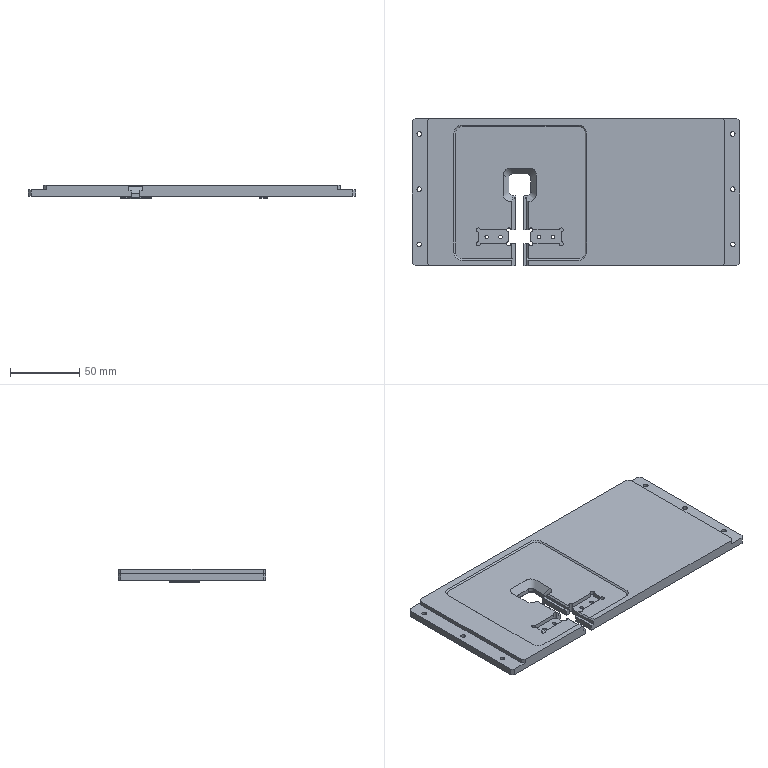NC program | NX | posted with a generic post | part box 237 x 107 x 9.5 mm
Lines 1 to 1380 of 4908:
N10 G17 G21 G94 G90
(CAVITY_MILL_COPY_1 , TOOL : D10)
N12 T20 M6
N14 G54
N16 G17 G0 G90 X9.751 Y58.449 S2800 M3
N18 G43 Z30. H20
N20 Z1.3
N22 G94 G1 Z-0.2 F1000.
N24 X12.147 Y54.299
N26 G3 X13.013 Y53.799 R1.
N28 G1 X118.5 F2200.
N30 G2 X118.799 Y53.499 R0.299
N32 G1 Y-53.499
N34 G2 X118.5 Y-53.799 R0.299
N36 G1 X-118.5
N38 G2 X-118.799 Y-53.499 R0.299
N40 G1 Y53.499
N42 G2 X-118.5 Y53.799 R0.299
N44 G1 X13.013
N46 Y46.799
N48 X111.799
N50 Y-46.799
N52 X-111.799
N54 Y46.799
N56 X13.013
N58 Y39.799
N60 X104.799
N62 Y-39.799
N64 X-104.799
N66 Y39.799
N68 X13.013
N70 Y32.799
N72 X97.799
N74 Y-32.799
N76 X-97.799
N78 Y32.799
N80 X13.013
N82 Y25.799
N84 X90.799
N86 Y-25.799
N88 X-90.799
N90 Y25.799
N92 X13.013
N94 Y18.799
N96 X83.799
N98 Y-18.799
N100 X-25.022
N102 G3 X-23.25 Y-13.3 R9.42
N104 G1 Y2.7
N106 G3 X-32.67 Y12.12 R9.42
N108 G1 X-37.602
N110 G3 X-40.669 Y11.343 R6.488
N112 X-43.736 Y12.12 R6.462
N114 G1 X-48.67
N116 G3 X-58.09 Y2.7 R9.42
N118 G1 Y-13.3
N120 G3 X-56.318 Y-18.799 R9.42
N122 G1 X-55.181 Y-17.981
N124 G2 X-56.69 Y-13.3 R8.02
N126 G1 Y2.7
N128 G2 X-48.67 Y10.72 R8.02
N130 G1 X-43.737
N132 G2 X-40.67 Y9.683 R5.062
N134 X-37.602 Y10.72 R5.088
N136 G1 X-32.67
N138 G2 X-24.65 Y2.7 R8.02
N140 G1 Y-13.3
N142 G2 X-32.67 Y-21.32 R8.02
N144 G1 X-48.67
N146 G2 X-55.181 Y-17.981 R8.02
N148 G1 X-56.318 Y-18.799
N150 X-83.799
N152 Y18.799
N154 X-62.338
N156 Y11.799
N158 G3 X-65.09 Y2.7 R16.42
N160 G1 Y-11.799
N162 X-76.799
N164 Y11.799
N166 X-62.338
N168 X-69.078 Y7.299
N170 G3 X-69.59 Y2.7 R20.92
N172 G1 Y-7.299
N174 X-72.299
N176 Y7.299
N178 X-69.078
N180 X-62.338 Y11.799
N182 Y18.799
N184 X13.013
N186 Y11.799
N188 X76.799
N190 Y-11.799
N192 X60.524
N194 G3 X60.907 Y-9.3 R8.347
N196 G1 Y-1.3
N198 G3 X60.22 Y2.017 R8.347
N200 G1 X66.643 Y4.799
N202 X69.799
N204 Y-4.799
N206 X67.907
N208 Y-1.3
N210 G3 X66.643 Y4.799 R15.347
N212 G1 X60.22 Y2.017
N214 G3 X52.56 Y7.047 R8.347
N216 G1 X50.56
N218 G3 X42.213 Y-1.3 R8.347
N220 G1 Y-9.3
N222 G3 X42.596 Y-11.799 R8.347
N224 G1 X43.931 Y-11.38
N226 G2 X43.613 Y-9.3 R6.947
N228 G1 Y-1.3
N230 G2 X50.56 Y5.647 R6.947
N232 G1 X52.56
N234 G2 X59.507 Y-1.3 R6.947
N236 G1 Y-9.3
N238 G2 X52.56 Y-16.247 R6.947
N240 G1 X50.56
N242 G2 X43.931 Y-11.38 R6.947
N244 G1 X42.596 Y-11.799
N246 X-16.25
N248 Y2.7
N250 G3 X-19.002 Y11.799 R16.42
N252 G1 X13.013
N254 Y4.799
N256 X36.477
N258 G3 X35.213 Y-1.3 R15.347
N260 G1 Y-4.799
N262 X-9.25
N264 Y2.7
N266 G3 X-9.345 Y4.799 R23.42
N268 G1 X13.013
N270 Y0.299
N272 X30.777
N274 G3 X30.738 Y-0.299 R19.847
N276 G1 X-4.75
N278 Y0.299
N280 X13.013
N282 G3 X13.879 Y0.799 R1.
N284 G1 Z1.3
N286 G0 Z30.
N288 X9.728 Y58.449
N290 Z1.1
N292 G1 Z-0.4 F1000.
N294 X12.124 Y54.299
N296 G3 X12.99 Y53.799 R1.
N298 G1 X118.5 F2200.
N300 G2 X118.799 Y53.5 R0.299
N302 G1 Y-53.5
N304 G2 X118.5 Y-53.799 R0.299
N306 G1 X-118.5
N308 G2 X-118.799 Y-53.5 R0.299
N310 G1 Y53.5
N312 G2 X-118.5 Y53.799 R0.299
N314 G1 X12.99
N316 Y46.799
N318 X111.799
N320 Y-46.799
N322 X-111.799
N324 Y46.799
N326 X12.99
N328 Y39.799
N330 X104.799
N332 Y-39.799
N334 X-104.799
N336 Y39.799
N338 X12.99
N340 Y32.799
N342 X97.799
N344 Y-32.799
N346 X-97.799
N348 Y32.799
N350 X12.99
N352 Y25.799
N354 X90.799
N356 Y-25.799
N358 X-90.799
N360 Y25.799
N362 X12.99
N364 Y18.799
N366 X83.799
N368 Y-18.799
N370 X-24.933
N372 G3 X-23.178 Y-13.3 R9.492
N374 G1 Y2.7
N376 G3 X-32.67 Y12.192 R9.492
N378 G1 X-37.663
N380 G3 X-40.672 Y11.444 R6.674
N382 X-43.678 Y12.192 R6.578
N384 G1 X-48.67
N386 G3 X-58.162 Y2.7 R9.492
N388 G1 Y-13.3
N390 G3 X-56.407 Y-18.799 R9.492
N392 G1 X-55.265 Y-17.988
N394 G2 X-56.762 Y-13.3 R8.092
N396 G1 Y2.7
N398 G2 X-48.67 Y10.792 R8.092
N400 G1 X-43.678
N402 G2 X-40.676 Y9.804 R5.178
N404 X-37.663 Y10.792 R5.274
N406 G1 X-32.67
N408 G2 X-24.578 Y2.7 R8.092
N410 G1 Y-13.3
N412 G2 X-32.67 Y-21.392 R8.092
N414 G1 X-48.67
N416 G2 X-55.265 Y-17.988 R8.092
N418 G1 X-56.407 Y-18.799
N420 X-83.799
N422 Y18.799
N424 X-62.424
N426 Y11.799
N428 G3 X-65.162 Y2.7 R16.492
N430 G1 Y-11.799
N432 X-76.799
N434 Y11.799
N436 X-62.424
N438 X-69.152 Y7.299
N440 G3 X-69.662 Y2.7 R20.992
N442 G1 Y-7.299
N444 X-72.299
N446 Y7.299
N448 X-69.152
N450 X-62.424 Y11.799
N452 Y18.799
N454 X12.99
N456 Y11.799
N458 X76.799
N460 Y-11.799
N462 X60.649
N464 G3 X61.026 Y-9.3 R8.466
N466 G1 Y-1.3
N468 G3 X60.34 Y2.038 R8.466
N470 G1 X66.772 Y4.799
N472 X69.799
N474 Y-4.799
N476 X68.026
N478 Y-1.3
N480 G3 X66.772 Y4.799 R15.466
N482 G1 X60.34 Y2.038
N484 G3 X52.56 Y7.166 R8.466
N486 G1 X50.56
N488 G3 X42.094 Y-1.3 R8.466
N490 G1 Y-9.3
N492 G3 X42.471 Y-11.799 R8.466
N494 G1 X43.809 Y-11.386
N496 G2 X43.494 Y-9.3 R7.066
N498 G1 Y-1.3
N500 G2 X50.56 Y5.766 R7.066
N502 G1 X52.56
N504 G2 X59.626 Y-1.3 R7.066
N506 G1 Y-9.3
N508 G2 X52.56 Y-16.366 R7.066
N510 G1 X50.56
N512 G2 X43.809 Y-11.386 R7.066
N514 G1 X42.471 Y-11.799
N516 X-16.178
N518 Y2.7
N520 G3 X-18.916 Y11.799 R16.492
N522 G1 X12.99
N524 Y4.799
N526 X36.348
N528 G3 X35.094 Y-1.3 R15.466
N530 G1 Y-4.799
N532 X-9.178
N534 Y2.7
N536 G3 X-9.272 Y4.799 R23.492
N538 G1 X12.99
N540 Y0.299
N542 X30.658
N544 G3 X30.619 Y-0.299 R19.966
N546 G1 X-4.678
N548 Y0.299
N550 X12.99
N552 G3 X13.856 Y0.799 R1.
N554 G1 Z1.1
N556 G0 Z30.
N558 X9.715 Y58.449
N560 Z0.9
N562 G1 Z-0.6 F1000.
N564 X12.111 Y54.299
N566 G3 X12.977 Y53.799 R1.
N568 G1 X118.5 F2200.
N570 G2 X118.799 Y53.5 R0.299
N572 G1 Y-53.5
N574 G2 X118.5 Y-53.799 R0.299
N576 G1 X-118.5
N578 G2 X-118.799 Y-53.5 R0.299
N580 G1 Y53.5
N582 G2 X-118.5 Y53.799 R0.299
N584 G1 X12.977
N586 Y46.799
N588 X111.799
N590 Y-46.799
N592 X-111.799
N594 Y46.799
N596 X12.977
N598 Y39.799
N600 X104.799
N602 Y-39.799
N604 X-104.799
N606 Y39.799
N608 X12.977
N610 Y32.799
N612 X97.799
N614 Y-32.799
N616 X-97.799
N618 Y32.799
N620 X12.977
N622 Y25.799
N624 X90.799
N626 Y-25.799
N628 X-90.799
N630 Y25.799
N632 X12.977
N634 Y18.799
N636 X83.799
N638 Y-18.799
N640 X-24.923
N642 G3 X-23.17 Y-13.3 R9.5
N644 G1 Y2.7
N646 G3 X-32.67 Y12.2 R9.5
N648 G1 X-37.676
N650 G3 X-40.67 Y11.466 R6.5
N652 X-43.67 Y12.2 R6.5
N654 G1 X-48.67
N656 G3 X-58.17 Y2.7 R9.5
N658 G1 Y-13.3
N660 G3 X-56.417 Y-18.799 R9.5
N662 G1 X-55.275 Y-17.988
N664 G2 X-56.77 Y-13.3 R8.1
N666 G1 Y2.7
N668 G2 X-48.67 Y10.8 R8.1
N670 G1 X-43.67
N672 G2 X-40.67 Y9.824 R5.1
N674 X-37.67 Y10.8 R5.1
N676 G1 X-32.67
N678 G2 X-24.57 Y2.7 R8.1
N680 G1 Y-13.3
N682 G2 X-32.67 Y-21.4 R8.1
N684 G1 X-48.67
N686 G2 X-55.275 Y-17.988 R8.1
N688 G1 X-56.417 Y-18.799
N690 X-83.799
N692 Y18.799
N694 X-62.435
N696 Y11.799
N698 G3 X-65.17 Y2.7 R16.5
N700 G1 Y-11.799
N702 X-76.799
N704 Y11.799
N706 X-62.435
N708 X-69.16 Y7.299
N710 G3 X-69.67 Y2.7 R21.
N712 G1 Y-7.299
N714 X-72.299
N716 Y7.299
N718 X-69.16
N720 X-62.435 Y11.799
N722 Y18.799
N724 X12.977
N726 Y11.799
N728 X76.799
N730 Y-11.799
N732 X60.684
N734 G3 X61.06 Y-9.33 R8.5
N736 G1 Y-1.27
N738 G3 X60.374 Y2.044 R8.5
N740 G1 X66.81 Y4.799
N742 X69.799
N744 Y-4.799
N746 X68.06
N748 Y-1.258
N750 G3 X66.81 Y4.799 R15.5
N752 G1 X60.374 Y2.044
N754 G3 X52.56 Y7.2 R8.5
N756 G1 X50.56
N758 G3 X42.06 Y-1.3 R8.5
N760 G1 Y-9.333
N762 G3 X42.436 Y-11.799 R8.5
N764 G1 X43.774 Y-11.387
N766 G2 X43.46 Y-9.3 R7.1
N768 G1 Y-1.3
N770 G2 X50.56 Y5.8 R7.1
N772 G1 X52.56
N774 G2 X59.66 Y-1.27 R7.1
N776 G1 Y-9.33
N778 G2 X52.56 Y-16.4 R7.1
N780 G1 X50.56
N782 G2 X43.774 Y-11.387 R7.1
N784 G1 X42.436 Y-11.799
N786 X-16.17
N788 Y2.7
N790 G3 X-18.905 Y11.799 R16.5
N792 G1 X12.977
N794 Y4.799
N796 X36.31
N798 G3 X35.06 Y-1.3 R15.5
N800 G1 Y-4.799
N802 X-9.17
N804 Y2.7
N806 G3 X-9.264 Y4.799 R23.5
N808 G1 X12.977
N810 Y0.299
N812 X30.624
N814 G3 X30.585 Y-0.299 R20.
N816 G1 X-4.67
N818 Y0.299
N820 X12.977
N822 G3 X13.843 Y0.799 R1.
N824 G1 Z0.9
N826 G0 Z30.
N828 X9.715 Y58.449
N830 Z0.7
N832 G1 Z-0.8 F1000.
N834 X12.111 Y54.299
N836 G3 X12.977 Y53.799 R1.
N838 G1 X118.5 F2200.
N840 G2 X118.799 Y53.5 R0.299
N842 G1 Y-53.5
N844 G2 X118.5 Y-53.799 R0.299
N846 G1 X-118.5
N848 G2 X-118.799 Y-53.5 R0.299
N850 G1 Y53.5
N852 G2 X-118.5 Y53.799 R0.299
N854 G1 X12.977
N856 Y46.799
N858 X111.799
N860 Y-46.799
N862 X-111.799
N864 Y46.799
N866 X12.977
N868 Y39.799
N870 X104.799
N872 Y-39.799
N874 X-104.799
N876 Y39.799
N878 X12.977
N880 Y32.799
N882 X97.799
N884 Y-32.799
N886 X-97.799
N888 Y32.799
N890 X12.977
N892 Y25.799
N894 X90.799
N896 Y-25.799
N898 X-90.799
N900 Y25.799
N902 X12.977
N904 Y18.799
N906 X83.799
N908 Y-18.799
N910 X-24.923
N912 G3 X-23.17 Y-13.3 R9.5
N914 G1 Y2.7
N916 G3 X-32.67 Y12.2 R9.5
N918 G1 X-37.676
N920 G3 X-40.67 Y11.466 R6.5
N922 X-43.67 Y12.2 R6.5
N924 G1 X-48.67
N926 G3 X-58.17 Y2.7 R9.5
N928 G1 Y-13.3
N930 G3 X-56.417 Y-18.799 R9.5
N932 G1 X-55.275 Y-17.988
N934 G2 X-56.77 Y-13.3 R8.1
N936 G1 Y2.7
N938 G2 X-48.67 Y10.8 R8.1
N940 G1 X-43.67
N942 G2 X-40.67 Y9.824 R5.1
N944 X-37.67 Y10.8 R5.1
N946 G1 X-32.67
N948 G2 X-24.57 Y2.7 R8.1
N950 G1 Y-13.3
N952 G2 X-32.67 Y-21.4 R8.1
N954 G1 X-48.67
N956 G2 X-55.275 Y-17.988 R8.1
N958 G1 X-56.417 Y-18.799
N960 X-83.799
N962 Y18.799
N964 X-62.435
N966 Y11.799
N968 G3 X-65.17 Y2.7 R16.5
N970 G1 Y-11.799
N972 X-76.799
N974 Y11.799
N976 X-62.435
N978 X-69.16 Y7.299
N980 G3 X-69.67 Y2.7 R21.
N982 G1 Y-7.299
N984 X-72.299
N986 Y7.299
N988 X-69.16
N990 X-62.435 Y11.799
N992 Y18.799
N994 X12.977
N996 Y11.799
N998 X76.799
N1000 Y-11.799
N1002 X60.684
N1004 G3 X61.06 Y-9.3 R8.5
N1006 G1 Y-1.3
N1008 G3 X60.374 Y2.044 R8.5
N1010 G1 X66.81 Y4.799
N1012 X69.799
N1014 Y-4.799
N1016 X68.06
N1018 Y-1.3
N1020 G3 X66.81 Y4.799 R15.5
N1022 G1 X60.374 Y2.044
N1024 G3 X52.56 Y7.2 R8.5
N1026 G1 X50.56
N1028 G3 X42.06 Y-1.3 R8.5
N1030 G1 Y-9.3
N1032 G3 X42.436 Y-11.799 R8.5
N1034 G1 X43.774 Y-11.387
N1036 G2 X43.46 Y-9.3 R7.1
N1038 G1 Y-1.3
N1040 G2 X50.56 Y5.8 R7.1
N1042 G1 X52.56
N1044 G2 X59.66 Y-1.3 R7.1
N1046 G1 Y-9.3
N1048 G2 X52.56 Y-16.4 R7.1
N1050 G1 X50.56
N1052 G2 X43.774 Y-11.387 R7.1
N1054 G1 X42.436 Y-11.799
N1056 X-16.17
N1058 Y2.7
N1060 G3 X-18.905 Y11.799 R16.5
N1062 G1 X12.977
N1064 Y4.799
N1066 X36.31
N1068 G3 X35.06 Y-1.3 R15.5
N1070 G1 Y-4.799
N1072 X-9.17
N1074 Y2.7
N1076 G3 X-9.264 Y4.799 R23.5
N1078 G1 X12.977
N1080 Y0.299
N1082 X30.624
N1084 G3 X30.585 Y-0.299 R20.
N1086 G1 X-4.67
N1088 Y0.299
N1090 X12.977
N1092 G3 X13.843 Y0.799 R1.
N1094 G1 Z0.7
N1096 G0 Z30.
N1098 X9.715 Y58.449
N1100 Z0.5
N1102 G1 Z-1. F1000.
N1104 X12.111 Y54.299
N1106 G3 X12.977 Y53.799 R1.
N1108 G1 X118.5 F2200.
N1110 G2 X118.799 Y53.5 R0.299
N1112 G1 Y-53.5
N1114 G2 X118.5 Y-53.799 R0.299
N1116 G1 X-118.5
N1118 G2 X-118.799 Y-53.5 R0.299
N1120 G1 Y53.5
N1122 G2 X-118.5 Y53.799 R0.299
N1124 G1 X12.977
N1126 Y46.799
N1128 X111.799
N1130 Y-46.799
N1132 X-111.799
N1134 Y46.799
N1136 X12.977
N1138 Y39.799
N1140 X104.799
N1142 Y-39.799
N1144 X-104.799
N1146 Y39.799
N1148 X12.977
N1150 Y32.799
N1152 X97.799
N1154 Y-32.799
N1156 X-97.799
N1158 Y32.799
N1160 X12.977
N1162 Y25.799
N1164 X90.799
N1166 Y-25.799
N1168 X-90.799
N1170 Y25.799
N1172 X12.977
N1174 Y18.799
N1176 X83.799
N1178 Y-18.799
N1180 X-24.923
N1182 G3 X-23.17 Y-13.3 R9.5
N1184 G1 Y2.7
N1186 G3 X-32.67 Y12.2 R9.5
N1188 G1 X-37.676
N1190 G3 X-40.67 Y11.466 R6.5
N1192 X-43.67 Y12.2 R6.5
N1194 G1 X-48.67
N1196 G3 X-58.17 Y2.7 R9.5
N1198 G1 Y-13.3
N1200 G3 X-56.417 Y-18.799 R9.5
N1202 G1 X-55.275 Y-17.988
N1204 G2 X-56.77 Y-13.3 R8.1
N1206 G1 Y2.7
N1208 G2 X-48.67 Y10.8 R8.1
N1210 G1 X-43.67
N1212 G2 X-40.67 Y9.824 R5.1
N1214 X-37.67 Y10.8 R5.1
N1216 G1 X-32.67
N1218 G2 X-24.57 Y2.7 R8.1
N1220 G1 Y-13.3
N1222 G2 X-32.67 Y-21.4 R8.1
N1224 G1 X-48.67
N1226 G2 X-55.275 Y-17.988 R8.1
N1228 G1 X-56.417 Y-18.799
N1230 X-83.799
N1232 Y18.799
N1234 X-62.435
N1236 Y11.799
N1238 G3 X-65.17 Y2.7 R16.5
N1240 G1 Y-11.799
N1242 X-76.799
N1244 Y11.799
N1246 X-62.435
N1248 X-69.16 Y7.299
N1250 G3 X-69.67 Y2.7 R21.
N1252 G1 Y-7.299
N1254 X-72.299
N1256 Y7.299
N1258 X-69.16
N1260 X-62.435 Y11.799
N1262 Y18.799
N1264 X12.977
N1266 Y11.799
N1268 X76.799
N1270 Y-11.799
N1272 X60.684
N1274 G3 X61.06 Y-9.3 R8.5
N1276 G1 Y-1.3
N1278 G3 X60.374 Y2.045 R8.5
N1280 G1 X66.81 Y4.799
N1282 X69.799
N1284 Y-4.799
N1286 X68.06
N1288 Y-1.3
N1290 G3 X66.81 Y4.799 R15.5
N1292 G1 X60.374 Y2.045
N1294 G3 X52.56 Y7.2 R8.5
N1296 G1 X50.56
N1298 G3 X42.06 Y-1.3 R8.5
N1300 G1 Y-9.3
N1302 G3 X42.436 Y-11.799 R8.5
N1304 G1 X43.774 Y-11.387
N1306 G2 X43.46 Y-9.3 R7.1
N1308 G1 Y-1.3
N1310 G2 X50.56 Y5.8 R7.1
N1312 G1 X52.56
N1314 G2 X59.66 Y-1.3 R7.1
N1316 G1 Y-9.3
N1318 G2 X52.56 Y-16.4 R7.1
N1320 G1 X50.56
N1322 G2 X43.774 Y-11.387 R7.1
N1324 G1 X42.436 Y-11.799
N1326 X-16.17
N1328 Y2.7
N1330 G3 X-18.905 Y11.799 R16.5
N1332 G1 X12.977
N1334 Y4.799
N1336 X36.31
N1338 G3 X35.06 Y-1.3 R15.5
N1340 G1 Y-4.799
N1342 X-9.17
N1344 Y2.7
N1346 G3 X-9.264 Y4.799 R23.5
N1348 G1 X12.977
N1350 Y0.299
N1352 X30.624
N1354 G3 X30.585 Y-0.299 R20.
N1356 G1 X-4.67
N1358 Y0.299
N1360 X12.977
N1362 G3 X13.843 Y0.799 R1.
N1364 G1 Z0.5
N1366 G0 Z30.
N1368 X9.715 Y58.449
N1370 Z0.3
N1372 G1 Z-1.2 F1000.
N1374 X12.111 Y54.299
N1376 G3 X12.977 Y53.799 R1.
N1378 G1 X118.5 F2200.
N1380 G2 X118.799 Y53.5 R0.299
N1382 G1 Y-53.5
N1384 G2 X118.5 Y-53.799 R0.299
N1386 G1 X-118.5
N1388 G2 X-118.799 Y-53.5 R0.299
N1390 G1 Y53.5
N1392 G2 X-118.5 Y53.799 R0.299
N1394 G1 X12.977
N1396 Y46.799
N1398 X111.799
N1400 Y-46.799
N1402 X-111.799
N1404 Y46.799
N1406 X12.977
N1408 Y39.799
N1410 X104.799
N1412 Y-39.799
N1414 X-104.799
N1416 Y39.799
N1418 X12.977
N1420 Y32.799
N1422 X97.799
N1424 Y-32.799
N1426 X-97.799
N1428 Y32.799
N1430 X12.977
N1432 Y25.799
N1434 X90.799
N1436 Y-25.799
N1438 X-90.799
N1440 Y25.799
N1442 X12.977
N1444 Y18.799
N1446 X83.799
N1448 Y-18.799
N1450 X-24.923
N1452 G3 X-23.17 Y-13.3 R9.5
N1454 G1 Y2.7
N1456 G3 X-32.67 Y12.2 R9.5
N1458 G1 X-37.676
N1460 G3 X-40.67 Y11.466 R6.5
N1462 X-43.67 Y12.2 R6.5
N1464 G1 X-48.67
N1466 G3 X-58.17 Y2.7 R9.5
N1468 G1 Y-13.3
N1470 G3 X-56.417 Y-18.799 R9.5
N1472 G1 X-55.275 Y-17.988
N1474 G2 X-56.77 Y-13.3 R8.1
N1476 G1 Y2.7
N1478 G2 X-48.67 Y10.8 R8.1
N1480 G1 X-43.67
N1482 G2 X-40.67 Y9.824 R5.1
N1484 X-37.67 Y10.8 R5.1
N1486 G1 X-32.67
N1488 G2 X-24.57 Y2.7 R8.1
N1490 G1 Y-13.3
N1492 G2 X-32.67 Y-21.4 R8.1
N1494 G1 X-48.67
N1496 G2 X-55.275 Y-17.988 R8.1
N1498 G1 X-56.417 Y-18.799
N1500 X-83.799
N1502 Y18.799
N1504 X-62.434
N1506 Y11.799
N1508 G3 X-65.17 Y2.7 R16.5
N1510 G1 Y-11.799
N1512 X-76.799
N1514 Y11.799
N1516 X-62.434
N1518 X-69.16 Y7.299
N1520 G3 X-69.67 Y2.7 R21.
N1522 G1 Y-7.299
N1524 X-72.299
N1526 Y7.299
N1528 X-69.16
N1530 X-62.434 Y11.799
N1532 Y18.799
N1534 X12.977
N1536 Y11.799
N1538 X76.799
N1540 Y-11.799
N1542 X60.684
N1544 G3 X61.06 Y-9.3 R8.5
N1546 G1 Y-1.3
N1548 G3 X60.374 Y2.045 R8.5
N1550 G1 X66.81 Y4.799
N1552 X69.799
N1554 Y-4.799
N1556 X68.06
N1558 Y-1.3
N1560 G3 X66.81 Y4.799 R15.5
N1562 G1 X60.374 Y2.045
N1564 G3 X52.56 Y7.2 R8.5
N1566 G1 X50.56
N1568 G3 X42.06 Y-1.3 R8.5
N1570 G1 Y-9.3
N1572 G3 X42.436 Y-11.799 R8.5
N1574 G1 X43.774 Y-11.387
N1576 G2 X43.46 Y-9.3 R7.1
N1578 G1 Y-1.3
N1580 G2 X50.56 Y5.8 R7.1
N1582 G1 X52.56
N1584 G2 X59.66 Y-1.3 R7.1
N1586 G1 Y-9.3
N1588 G2 X52.56 Y-16.4 R7.1
N1590 G1 X50.56
N1592 G2 X43.774 Y-11.387 R7.1
N1594 G1 X42.436 Y-11.799
N1596 X-16.17
N1598 Y2.7
N1600 G3 X-18.906 Y11.799 R16.5
N1602 G1 X12.977
N1604 Y4.799
N1606 X36.31
N1608 G3 X35.06 Y-1.3 R15.5
N1610 G1 Y-4.799
N1612 X-9.17
N1614 Y2.7
N1616 G3 X-9.264 Y4.799 R23.5
N1618 G1 X12.977
N1620 Y0.299
N1622 X30.624
N1624 G3 X30.585 Y-0.299 R20.
N1626 G1 X-4.67
N1628 Y0.299
N1630 X12.977
N1632 G3 X13.843 Y0.799 R1.
N1634 G1 Z0.3
N1636 G0 Z30.
N1638 X9.715 Y58.449
N1640 Z0.1
N1642 G1 Z-1.4 F1000.
N1644 X12.111 Y54.299
N1646 G3 X12.977 Y53.799 R1.
N1648 G1 X118.5 F2200.
N1650 G2 X118.799 Y53.5 R0.299
N1652 G1 Y-53.5
N1654 G2 X118.5 Y-53.799 R0.299
N1656 G1 X-118.5
N1658 G2 X-118.799 Y-53.5 R0.299
N1660 G1 Y53.5
N1662 G2 X-118.5 Y53.799 R0.299
N1664 G1 X12.977
N1666 Y46.799
N1668 X111.799
N1670 Y-46.799
N1672 X-111.799
N1674 Y46.799
N1676 X12.977
N1678 Y39.799
N1680 X104.799
N1682 Y-39.799
N1684 X-104.799
N1686 Y39.799
N1688 X12.977
N1690 Y32.799
N1692 X97.799
N1694 Y-32.799
N1696 X-97.799
N1698 Y32.799
N1700 X12.977
N1702 Y25.799
N1704 X90.799
N1706 Y-25.799
N1708 X-90.799
N1710 Y25.799
N1712 X12.977
N1714 Y18.799
N1716 X83.799
N1718 Y-18.799
N1720 X-24.923
N1722 G3 X-23.17 Y-13.3 R9.5
N1724 G1 Y2.7
N1726 G3 X-32.67 Y12.2 R9.5
N1728 G1 X-37.676
N1730 G3 X-40.67 Y11.466 R6.5
N1732 X-43.67 Y12.2 R6.5
N1734 G1 X-48.67
N1736 G3 X-58.17 Y2.7 R9.5
N1738 G1 Y-13.3
N1740 G3 X-56.417 Y-18.799 R9.5
N1742 G1 X-55.275 Y-17.988
N1744 G2 X-56.77 Y-13.3 R8.1
N1746 G1 Y2.7
N1748 G2 X-48.67 Y10.8 R8.1
N1750 G1 X-43.67
N1752 G2 X-40.67 Y9.824 R5.1
N1754 X-37.67 Y10.8 R5.1
N1756 G1 X-32.67
N1758 G2 X-24.57 Y2.7 R8.1
N1760 G1 Y-13.3
N1762 G2 X-32.67 Y-21.4 R8.1
N1764 G1 X-48.67
N1766 G2 X-55.275 Y-17.988 R8.1
N1768 G1 X-56.417 Y-18.799
N1770 X-83.799
N1772 Y18.799
N1774 X-62.434
N1776 Y11.799
N1778 G3 X-65.17 Y2.7 R16.5
N1780 G1 Y-11.799
N1782 X-76.799
N1784 Y11.799
N1786 X-62.434
N1788 X-69.16 Y7.299
N1790 G3 X-69.67 Y2.7 R21.
N1792 G1 Y-7.299
N1794 X-72.299
N1796 Y7.299
N1798 X-69.16
N1800 X-62.434 Y11.799
N1802 Y18.799
N1804 X12.977
N1806 Y11.799
N1808 X76.799
N1810 Y-11.799
N1812 X60.684
N1814 G3 X61.06 Y-9.3 R8.5
N1816 G1 Y-1.3
N1818 G3 X60.374 Y2.045 R8.5
N1820 G1 X66.81 Y4.799
N1822 X69.799
N1824 Y-4.799
N1826 X68.06
N1828 Y-1.3
N1830 G3 X66.81 Y4.799 R15.5
N1832 G1 X60.374 Y2.045
N1834 G3 X52.56 Y7.2 R8.5
N1836 G1 X50.56
N1838 G3 X42.06 Y-1.3 R8.5
N1840 G1 Y-9.3
N1842 G3 X42.436 Y-11.799 R8.5
N1844 G1 X43.774 Y-11.387
N1846 G2 X43.46 Y-9.3 R7.1
N1848 G1 Y-1.3
N1850 G2 X50.56 Y5.8 R7.1
N1852 G1 X52.56
N1854 G2 X59.66 Y-1.3 R7.1
N1856 G1 Y-9.3
N1858 G2 X52.56 Y-16.4 R7.1
N1860 G1 X50.56
N1862 G2 X43.774 Y-11.387 R7.1
N1864 G1 X42.436 Y-11.799
N1866 X-16.17
N1868 Y2.7
N1870 G3 X-18.906 Y11.799 R16.5
N1872 G1 X12.977
N1874 Y4.799
N1876 X36.31
N1878 G3 X35.06 Y-1.3 R15.5
N1880 G1 Y-4.799
N1882 X-9.17
N1884 Y2.7
N1886 G3 X-9.264 Y4.799 R23.5
N1888 G1 X12.977
N1890 Y0.299
N1892 X30.624
N1894 G3 X30.585 Y-0.299 R20.
N1896 G1 X-4.67
N1898 Y0.299
N1900 X12.977
N1902 G3 X13.843 Y0.799 R1.
N1904 G1 Z0.1
N1906 G0 Z30.
(CAVITY_MILL_COPY_1_COPY , TOOL : D10)
N1908 X8.135 Y-5.161
N1910 Z0.
N1912 G1 X-4.769 Z-0.676 F1000.
N1914 Y-5.439 Z-0.691
N1916 X14.87 Z-1.72
N1918 X34.509 F2200.
N1920 Y-5.161
N1922 X-4.769
N1924 Y-5.439
N1926 X14.87
N1928 Y-12.439
N1930 X41.509
N1932 Y1.839
N1934 X-11.769
N1936 Y-12.439
N1938 X14.87
N1940 G3 X15.736 Y-11.939 R1.
N1942 G1 Z-0.22
N1944 G0 Z30.
N1946 X-0.99 Y-2.88
N1948 Z-0.22
N1950 G1 X-7.05 Z-0.538 F1000.
N1952 Y-7.72 Z-0.791
N1954 X14.87 Z-1.94
N1956 X36.79 F2200.
N1958 Y-2.88
N1960 X-7.05
N1962 Y-7.72
N1964 X14.87
N1966 Y-12.22
N1968 X41.29
N1970 Y1.62
N1972 X-11.55
N1974 Y-12.22
N1976 X14.87
N1978 G3 X15.736 Y-11.72 R1.
N1980 G1 Z-0.44
N1982 G0 Z30.
N1984 X-0.91 Y-2.9
N1986 Z-0.44
N1988 G1 X-7.03 Z-0.761 F1000.
N1990 Y-7.7 Z-1.012
N1992 X14.87 Z-2.16
N1994 X36.77 F2200.
N1996 Y-2.9
N1998 X-7.03
N2000 Y-7.7
N2002 X14.87
N2004 Y-12.2
N2006 X41.27
N2008 Y1.6
N2010 X-11.53
N2012 Y-12.2
N2014 X14.87
N2016 G3 X15.736 Y-11.7 R1.
N2018 G1 Z-0.66
N2020 G0 Z30.
N2022 X-0.91 Y-2.9
N2024 Z-0.66
N2026 G1 X-7.03 Z-0.981 F1000.
N2028 Y-7.7 Z-1.232
N2030 X14.87 Z-2.38
N2032 X36.77 F2200.
N2034 Y-2.9
N2036 X-7.03
N2038 Y-7.7
N2040 X14.87
N2042 Y-12.2
N2044 X41.27
N2046 Y1.6
N2048 X-11.53
N2050 Y-12.2
N2052 X14.87
N2054 G3 X15.736 Y-11.7 R1.
N2056 G1 Z-0.88
N2058 G0 Z30.
N2060 X-0.91 Y-2.9
N2062 Z-0.88
N2064 G1 X-7.03 Z-1.201 F1000.
N2066 Y-7.7 Z-1.452
N2068 X14.87 Z-2.6
N2070 X36.77 F2200.
N2072 Y-2.9
N2074 X-7.03
N2076 Y-7.7
N2078 X14.87
N2080 Y-12.2
N2082 X41.27
N2084 Y1.6
N2086 X-11.53
N2088 Y-12.2
N2090 X14.87
N2092 G3 X15.736 Y-11.7 R1.
N2094 G1 Z-1.1
N2096 G0 Z30.
N2098 X-0.91 Y-2.9
N2100 Z-1.1
N2102 G1 X-7.03 Z-1.421 F1000.
N2104 Y-7.7 Z-1.672
N2106 X14.87 Z-2.82
N2108 X36.77 F2200.
N2110 Y-2.9
N2112 X-7.03
N2114 Y-7.7
N2116 X14.87
N2118 Y-12.2
N2120 X41.27
N2122 Y1.6
N2124 X-11.53
N2126 Y-12.2
N2128 X14.87
N2130 G3 X15.736 Y-11.7 R1.
N2132 G1 Z-1.32
N2134 G0 Z30.
N2136 X-0.91 Y-2.9
N2138 Z-1.32
N2140 G1 X-7.03 Z-1.641 F1000.
N2142 Y-7.7 Z-1.892
N2144 X14.87 Z-3.04
N2146 X36.77 F2200.
N2148 Y-2.9
N2150 X-7.03
N2152 Y-7.7
N2154 X14.87
N2156 Y-12.2
N2158 X41.27
N2160 Y1.6
N2162 X-11.53
N2164 Y-12.2
N2166 X14.87
N2168 G3 X15.736 Y-11.7 R1.
N2170 G1 Z-1.54
N2172 G0 X-0.91 Y-2.9
N2174 G1 X-7.03 Z-1.861 F1000.
N2176 Y-7.7 Z-2.112
N2178 X14.87 Z-3.26
N2180 X36.77 F2200.
N2182 Y-2.9
N2184 X-7.03
N2186 Y-7.7
N2188 X14.87
N2190 Y-12.2
N2192 X41.27
N2194 Y1.6
N2196 X-11.53
N2198 Y-12.2
N2200 X14.87
N2202 G3 X15.736 Y-11.7 R1.
N2204 G1 Z-1.76
N2206 G0 X-0.91 Y-2.9
N2208 G1 X-7.03 Z-2.081 F1000.
N2210 Y-7.7 Z-2.332
N2212 X14.87 Z-3.48
N2214 X36.77 F2200.
N2216 Y-2.9
N2218 X-7.03
N2220 Y-7.7
N2222 X14.87
N2224 Y-12.2
N2226 X41.27
N2228 Y1.6
N2230 X-11.53
N2232 Y-12.2
N2234 X14.87
N2236 G3 X15.736 Y-11.7 R1.
N2238 G1 Z-1.98
N2240 G0 X-0.91 Y-2.9
N2242 G1 X-7.03 Z-2.301 F1000.
N2244 Y-7.7 Z-2.552
N2246 X14.87 Z-3.7
N2248 X36.77 F2200.
N2250 Y-2.9
N2252 X-7.03
N2254 Y-7.7
N2256 X14.87
N2258 Y-12.2
N2260 X41.27
N2262 Y1.6
N2264 X-11.53
N2266 Y-12.2
N2268 X14.87
N2270 G3 X15.736 Y-11.7 R1.
N2272 G1 Z-2.2
N2274 G0 X-0.91 Y-2.9
N2276 G1 X-7.03 Z-2.521 F1000.
N2278 Y-7.7 Z-2.772
N2280 X14.87 Z-3.92
N2282 X36.77 F2200.
N2284 Y-2.9
N2286 X-7.03
N2288 Y-7.7
N2290 X14.87
N2292 Y-12.2
N2294 X41.27
N2296 Y1.6
N2298 X-11.53
N2300 Y-12.2
N2302 X14.87
N2304 G3 X15.736 Y-11.7 R1.
N2306 G1 Z-2.42
N2308 G0 X-0.91 Y-2.9
N2310 G1 X-7.03 Z-2.741 F1000.
N2312 Y-7.7 Z-2.992
N2314 X14.87 Z-4.14
N2316 X36.77 F2200.
N2318 Y-2.9
N2320 X-7.03
N2322 Y-7.7
N2324 X14.87
N2326 Y-12.2
N2328 X41.27
N2330 Y1.6
N2332 X-11.53
N2334 Y-12.2
N2336 X14.87
N2338 G3 X15.736 Y-11.7 R1.
N2340 G1 Z-2.64
N2342 G0 X-0.91 Y-2.9
N2344 G1 X-7.03 Z-2.961 F1000.
N2346 Y-7.7 Z-3.212
N2348 X14.87 Z-4.36
N2350 X36.77 F2200.
N2352 Y-2.9
N2354 X-7.03
N2356 Y-7.7
N2358 X14.87
N2360 Y-12.2
N2362 X41.27
N2364 Y1.6
N2366 X-11.53
N2368 Y-12.2
N2370 X14.87
N2372 G3 X15.736 Y-11.7 R1.
N2374 G1 Z-2.86
N2376 G0 X-0.91 Y-2.9
N2378 G1 X-7.03 Z-3.181 F1000.
N2380 Y-7.7 Z-3.432
N2382 X14.87 Z-4.58
N2384 X36.77 F2200.
N2386 Y-2.9
N2388 X-7.03
N2390 Y-7.7
N2392 X14.87
N2394 Y-12.2
N2396 X41.27
N2398 Y1.6
N2400 X-11.53
N2402 Y-12.2
N2404 X14.87
N2406 G3 X15.736 Y-11.7 R1.
N2408 G1 Z-3.08
N2410 G0 X-0.91 Y-2.9
N2412 G1 X-7.03 Z-3.401 F1000.
N2414 Y-7.7 Z-3.652
N2416 X14.87 Z-4.8
N2418 X36.77 F2200.
N2420 Y-2.9
N2422 X-7.03
N2424 Y-7.7
N2426 X14.87
N2428 Y-12.2
N2430 X41.27
N2432 Y1.6
N2434 X-11.53
N2436 Y-12.2
N2438 X14.87
N2440 G3 X15.736 Y-11.7 R1.
N2442 G1 Z-3.3
N2444 G0 X-0.91 Y-2.9
N2446 G1 X-7.03 Z-3.621 F1000.
N2448 Y-7.7 Z-3.872
N2450 X14.87 Z-5.02
N2452 X36.77 F2200.
N2454 Y-2.9
N2456 X-7.03
N2458 Y-7.7
N2460 X14.87
N2462 Y-12.2
N2464 X41.27
N2466 Y1.6
N2468 X-11.53
N2470 Y-12.2
N2472 X14.87
N2474 G3 X15.736 Y-11.7 R1.
N2476 G1 Z-3.52
N2478 G0 X-0.91 Y-2.9
N2480 G1 X-7.03 Z-3.841 F1000.
N2482 Y-7.7 Z-4.092
N2484 X14.87 Z-5.24
N2486 X36.77 F2200.
N2488 Y-2.9
N2490 X-7.03
N2492 Y-7.7
N2494 X14.87
N2496 Y-12.2
N2498 X41.27
N2500 Y1.6
N2502 X-11.53
N2504 Y-12.2
N2506 X14.87
N2508 G3 X15.736 Y-11.7 R1.
N2510 G1 Z-3.74
N2512 G0 X-0.91 Y-2.9
N2514 G1 X-7.03 Z-4.061 F1000.
N2516 Y-7.7 Z-4.312
N2518 X14.87 Z-5.46
N2520 X36.77 F2200.
N2522 Y-2.9
N2524 X-7.03
N2526 Y-7.7
N2528 X14.87
N2530 Y-12.2
N2532 X41.27
N2534 Y1.6
N2536 X-11.53
N2538 Y-12.2
N2540 X14.87
N2542 G3 X15.736 Y-11.7 R1.
N2544 G1 Z-3.96
N2546 G0 X-0.91 Y-2.9
N2548 G1 X-7.03 Z-4.281 F1000.
N2550 Y-7.7 Z-4.532
N2552 X14.87 Z-5.68
N2554 X36.77 F2200.
N2556 Y-2.9
N2558 X-7.03
N2560 Y-7.7
N2562 X14.87
N2564 Y-12.2
N2566 X41.27
N2568 Y1.6
N2570 X-11.53
N2572 Y-12.2
N2574 X14.87
N2576 G3 X15.736 Y-11.7 R1.
N2578 G1 Z-4.18
N2580 G0 X-0.91 Y-2.9
N2582 G1 X-7.03 Z-4.501 F1000.
N2584 Y-7.7 Z-4.752
N2586 X14.87 Z-5.9
N2588 X36.77 F2200.
N2590 Y-2.9
N2592 X-7.03
N2594 Y-7.7
N2596 X14.87
N2598 Y-12.2
N2600 X41.27
N2602 Y1.6
N2604 X-11.53
N2606 Y-12.2
N2608 X14.87
N2610 G3 X15.736 Y-11.7 R1.
N2612 G1 Z-4.4
N2614 G0 X-0.91 Y-2.9
N2616 G1 X-7.03 Z-4.721 F1000.
N2618 Y-7.7 Z-4.972
N2620 X14.87 Z-6.12
N2622 X36.77 F2200.
N2624 Y-2.9
N2626 X-7.03
N2628 Y-7.7
N2630 X14.87
N2632 Y-12.2
N2634 X41.27
N2636 Y1.6
N2638 X-11.53
N2640 Y-12.2
N2642 X14.87
N2644 G3 X15.736 Y-11.7 R1.
N2646 G1 Z-4.62
N2648 G0 X-0.91 Y-2.9
N2650 G1 X-7.03 Z-4.941 F1000.
N2652 Y-7.7 Z-5.192
N2654 X14.87 Z-6.34
N2656 X36.77 F2200.
N2658 Y-2.9
N2660 X-7.03
N2662 Y-7.7
N2664 X14.87
N2666 Y-12.2
N2668 X41.27
N2670 Y1.6
N2672 X-11.53
N2674 Y-12.2
N2676 X14.87
N2678 G3 X15.736 Y-11.7 R1.
N2680 G1 Z-4.84
N2682 G0 X-0.91 Y-2.9
N2684 G1 X-7.03 Z-5.161 F1000.
N2686 Y-7.7 Z-5.412
N2688 X14.87 Z-6.56
N2690 X36.77 F2200.
N2692 Y-2.9
N2694 X-7.03
N2696 Y-7.7
N2698 X14.87
N2700 Y-12.2
N2702 X41.27
N2704 Y1.6
N2706 X-11.53
N2708 Y-12.2
N2710 X14.87
N2712 G3 X15.736 Y-11.7 R1.
N2714 G1 Z-5.06
N2716 G0 X-0.91 Y-2.9
N2718 G1 X-7.03 Z-5.381 F1000.
N2720 Y-7.7 Z-5.632
N2722 X14.87 Z-6.78
N2724 X36.77 F2200.
N2726 Y-2.9
N2728 X-7.03
N2730 Y-7.7
N2732 X14.87
N2734 Y-12.2
N2736 X41.27
N2738 Y1.6
N2740 X-11.53
N2742 Y-12.2
N2744 X14.87
N2746 G3 X15.736 Y-11.7 R1.
N2748 G1 Z-5.28
N2750 G0 Z30.
N2752 M5